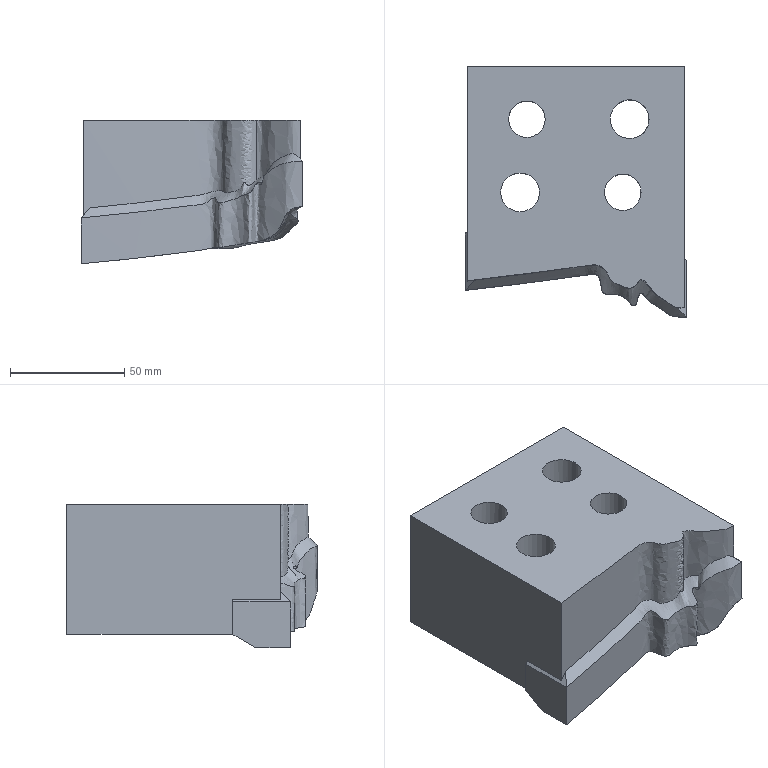Part | NX | features solid 2 | 1 solid | 37 faces | box 97 x 109.653 x 62.827 mm | volume 416609 mm3 | spline 21 | plane 10 | cylinder 6 | commonest cylinder face diameters 16 x2 17 x2 25 x2